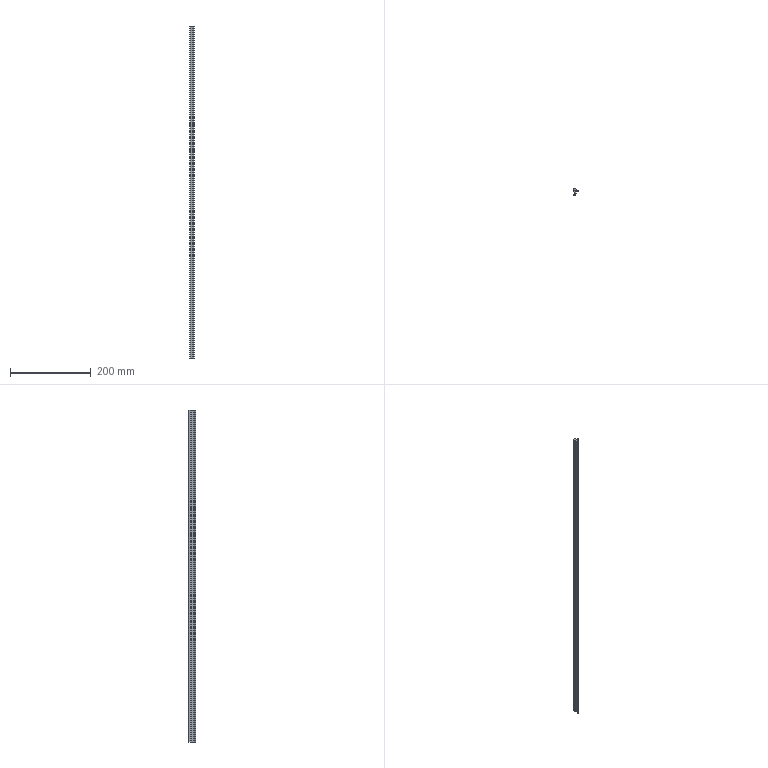Part | SolidWorks | features BaseBody 1, MoveFace 1 | 1 solid | 20 faces | box 10.8 x 17.5 x 820 mm | volume 64616 mm3 | cylinder 11 | plane 9 | commonest cylinder face diameters 1.6 x2 14 x2 0.4 x1 0.6 x1 0.8 x1 2.6 x1
STEP:
#1=CARTESIAN_POINT('',(-3.236,-11.055,720.));
#2=VERTEX_POINT('',#1);
#3=CARTESIAN_POINT('',(-4.3,-10.3,720.));
#4=VERTEX_POINT('',#3);
#5=CARTESIAN_POINT('',(-3.5,-10.3,720.));
#6=DIRECTION('',(0.,0.,-1.));
#7=DIRECTION('',(1.,0.,0.));
#8=AXIS2_PLACEMENT_3D('',#5,#6,#7);
#9=CIRCLE('',#8,0.8);
#10=EDGE_CURVE('',#2,#4,#9,.T.);
#11=ORIENTED_EDGE('',*,*,#10,.T.);
#12=CARTESIAN_POINT('',(-4.3,-10.3,-100.));
#13=VERTEX_POINT('',#12);
#14=CARTESIAN_POINT('',(-4.3,-10.3,-100.));
#15=DIRECTION('',(0.,0.,-1.));
#16=VECTOR('',#15,1000.);
#17=LINE('',#14,#16);
#18=EDGE_CURVE('',#4,#13,#17,.T.);
#19=ORIENTED_EDGE('',*,*,#18,.T.);
#20=CARTESIAN_POINT('',(-3.236,-11.055,-100.));
#21=VERTEX_POINT('',#20);
#22=CARTESIAN_POINT('',(-3.5,-10.3,-100.));
#23=DIRECTION('',(0.,0.,1.));
#24=DIRECTION('',(-1.,0.,0.));
#25=AXIS2_PLACEMENT_3D('',#22,#23,#24);
#26=CIRCLE('',#25,0.8);
#27=EDGE_CURVE('',#13,#21,#26,.T.);
#28=ORIENTED_EDGE('',*,*,#27,.T.);
#29=CARTESIAN_POINT('',(-3.236,-11.055,-100.));
#30=DIRECTION('',(0.,0.,-1.));
#31=VECTOR('',#30,1000.);
#32=LINE('',#29,#31);
#33=EDGE_CURVE('',#2,#21,#32,.T.);
#34=ORIENTED_EDGE('',*,*,#33,.F.);
#35=EDGE_LOOP('',(#11,#19,#28,#34));
#36=FACE_OUTER_BOUND('',#35,.T.);
#37=CARTESIAN_POINT('',(-3.5,-10.3,-100.));
#38=DIRECTION('',(0.,0.,-1.));
#39=DIRECTION('',(-1.,0.,0.));
#40=AXIS2_PLACEMENT_3D('',#37,#38,#39);
#41=CYLINDRICAL_SURFACE('',#40,0.8);
#42=ADVANCED_FACE('',(#36),#41,.T.);
#43=CARTESIAN_POINT('',(1.184,-6.397,-100.));
#44=VERTEX_POINT('',#43);
#45=CARTESIAN_POINT('',(-5.702,-4.29,-100.));
#46=DIRECTION('',(0.,0.,1.));
#47=DIRECTION('',(-1.,0.,0.));
#48=AXIS2_PLACEMENT_3D('',#45,#46,#47);
#49=CIRCLE('',#48,7.201);
#50=EDGE_CURVE('',#21,#44,#49,.T.);
#51=ORIENTED_EDGE('',*,*,#50,.T.);
#52=CARTESIAN_POINT('',(1.184,-6.397,720.));
#53=VERTEX_POINT('',#52);
#54=CARTESIAN_POINT('',(1.184,-6.397,-100.));
#55=DIRECTION('',(0.,0.,1.));
#56=VECTOR('',#55,1000.);
#57=LINE('',#54,#56);
#58=EDGE_CURVE('',#44,#53,#57,.T.);
#59=ORIENTED_EDGE('',*,*,#58,.T.);
#60=CARTESIAN_POINT('',(-5.702,-4.29,720.));
#61=DIRECTION('',(0.,0.,-1.));
#62=DIRECTION('',(1.,0.,0.));
#63=AXIS2_PLACEMENT_3D('',#60,#61,#62);
#64=CIRCLE('',#63,7.201);
#65=EDGE_CURVE('',#53,#2,#64,.T.);
#66=ORIENTED_EDGE('',*,*,#65,.T.);
#67=ORIENTED_EDGE('',*,*,#33,.T.);
#68=EDGE_LOOP('',(#51,#59,#66,#67));
#69=FACE_OUTER_BOUND('',#68,.T.);
#70=CARTESIAN_POINT('',(-5.702,-4.29,-100.));
#71=DIRECTION('',(0.,0.,-1.));
#72=DIRECTION('',(-1.,0.,0.));
#73=AXIS2_PLACEMENT_3D('',#70,#71,#72);
#74=CYLINDRICAL_SURFACE('',#73,7.201);
#75=ADVANCED_FACE('',(#69),#74,.T.);
#76=CARTESIAN_POINT('',(0.9,-6.,-100.));
#77=VERTEX_POINT('',#76);
#78=CARTESIAN_POINT('',(0.9,-6.3,-100.));
#79=DIRECTION('',(0.,0.,1.));
#80=DIRECTION('',(-1.,0.,0.));
#81=AXIS2_PLACEMENT_3D('',#78,#79,#80);
#82=CIRCLE('',#81,0.3);
#83=EDGE_CURVE('',#44,#77,#82,.T.);
#84=ORIENTED_EDGE('',*,*,#83,.T.);
#85=CARTESIAN_POINT('',(0.9,-6.,720.));
#86=VERTEX_POINT('',#85);
#87=CARTESIAN_POINT('',(0.9,-6.,-100.));
#88=DIRECTION('',(0.,0.,1.));
#89=VECTOR('',#88,1000.);
#90=LINE('',#87,#89);
#91=EDGE_CURVE('',#77,#86,#90,.T.);
#92=ORIENTED_EDGE('',*,*,#91,.T.);
#93=CARTESIAN_POINT('',(0.9,-6.3,720.));
#94=DIRECTION('',(0.,0.,-1.));
#95=DIRECTION('',(1.,0.,0.));
#96=AXIS2_PLACEMENT_3D('',#93,#94,#95);
#97=CIRCLE('',#96,0.3);
#98=EDGE_CURVE('',#86,#53,#97,.T.);
#99=ORIENTED_EDGE('',*,*,#98,.T.);
#100=ORIENTED_EDGE('',*,*,#58,.F.);
#101=EDGE_LOOP('',(#84,#92,#99,#100));
#102=FACE_OUTER_BOUND('',#101,.T.);
#103=CARTESIAN_POINT('',(0.9,-6.3,-100.));
#104=DIRECTION('',(0.,0.,-1.));
#105=DIRECTION('',(-1.,0.,0.));
#106=AXIS2_PLACEMENT_3D('',#103,#104,#105);
#107=CYLINDRICAL_SURFACE('',#106,0.3);
#108=ADVANCED_FACE('',(#102),#107,.T.);
#109=CARTESIAN_POINT('',(-2.5,-0.5,-100.));
#110=VERTEX_POINT('',#109);
#111=CARTESIAN_POINT('',(-2.5,-6.153,-100.));
#112=VERTEX_POINT('',#111);
#113=CARTESIAN_POINT('',(-2.5,-6.397,-100.));
#114=DIRECTION('',(0.,-1.,0.));
#115=VECTOR('',#114,1000.);
#116=LINE('',#113,#115);
#117=EDGE_CURVE('',#110,#112,#116,.T.);
#118=ORIENTED_EDGE('',*,*,#117,.F.);
#119=CARTESIAN_POINT('',(-4.2,1.695,-100.));
#120=VERTEX_POINT('',#119);
#121=CARTESIAN_POINT('',(-1.701,1.875,-100.));
#122=DIRECTION('',(0.,0.,1.));
#123=DIRECTION('',(-1.,0.,0.));
#124=AXIS2_PLACEMENT_3D('',#121,#122,#123);
#125=CIRCLE('',#124,2.506);
#126=EDGE_CURVE('',#120,#110,#125,.T.);
#127=ORIENTED_EDGE('',*,*,#126,.F.);
#128=CARTESIAN_POINT('',(-4.2,5.1,-100.));
#129=VERTEX_POINT('',#128);
#130=CARTESIAN_POINT('',(-4.2,-6.397,-100.));
#131=DIRECTION('',(0.,-1.,0.));
#132=VECTOR('',#131,1000.);
#133=LINE('',#130,#132);
#134=EDGE_CURVE('',#129,#120,#133,.T.);
#135=ORIENTED_EDGE('',*,*,#134,.F.);
#136=CARTESIAN_POINT('',(-2.892,6.4,-100.));
#137=VERTEX_POINT('',#136);
#138=CARTESIAN_POINT('',(-2.9,5.1,-100.));
#139=DIRECTION('',(0.,0.,1.));
#140=DIRECTION('',(-1.,0.,0.));
#141=AXIS2_PLACEMENT_3D('',#138,#139,#140);
#142=CIRCLE('',#141,1.3);
#143=EDGE_CURVE('',#137,#129,#142,.T.);
#144=ORIENTED_EDGE('',*,*,#143,.F.);
#145=CARTESIAN_POINT('',(0.5,5.5,-100.));
#146=VERTEX_POINT('',#145);
#147=CARTESIAN_POINT('',(-2.934,-0.5999,-100.));
#148=DIRECTION('',(0.,0.,1.));
#149=DIRECTION('',(-1.,0.,0.));
#150=AXIS2_PLACEMENT_3D('',#147,#148,#149);
#151=CIRCLE('',#150,7.);
#152=EDGE_CURVE('',#146,#137,#151,.T.);
#153=ORIENTED_EDGE('',*,*,#152,.F.);
#154=CARTESIAN_POINT('',(5.5,1.7,-100.));
#155=VERTEX_POINT('',#154);
#156=CARTESIAN_POINT('',(5.5,1.7,-100.));
#157=DIRECTION('',(-0.7962,0.6051,0.));
#158=VECTOR('',#157,1000.);
#159=LINE('',#156,#158);
#160=EDGE_CURVE('',#155,#146,#159,.T.);
#161=ORIENTED_EDGE('',*,*,#160,.F.);
#162=CARTESIAN_POINT('',(6.458,-0.2215,-100.));
#163=VERTEX_POINT('',#162);
#164=CARTESIAN_POINT('',(6.458,-0.2215,-100.));
#165=DIRECTION('',(-0.4462,0.8949,0.));
#166=VECTOR('',#165,1000.);
#167=LINE('',#164,#166);
#168=EDGE_CURVE('',#163,#155,#167,.T.);
#169=ORIENTED_EDGE('',*,*,#168,.F.);
#170=CARTESIAN_POINT('',(5.895,-0.7433,-100.));
#171=VERTEX_POINT('',#170);
#172=CARTESIAN_POINT('',(6.1,-0.4,-100.));
#173=DIRECTION('',(0.,0.,1.));
#174=DIRECTION('',(-1.,0.,0.));
#175=AXIS2_PLACEMENT_3D('',#172,#173,#174);
#176=CIRCLE('',#175,0.4);
#177=EDGE_CURVE('',#171,#163,#176,.T.);
#178=ORIENTED_EDGE('',*,*,#177,.F.);
#179=CARTESIAN_POINT('',(3.,0.,-100.));
#180=VERTEX_POINT('',#179);
#181=CARTESIAN_POINT('',(2.746,-6.995,-100.));
#182=DIRECTION('',(0.,0.,-1.));
#183=DIRECTION('',(-1.,0.,0.));
#184=AXIS2_PLACEMENT_3D('',#181,#182,#183);
#185=CIRCLE('',#184,7.);
#186=EDGE_CURVE('',#180,#171,#185,.T.);
#187=ORIENTED_EDGE('',*,*,#186,.F.);
#188=CARTESIAN_POINT('',(0.,0.,-100.));
#189=VERTEX_POINT('',#188);
#190=CARTESIAN_POINT('',(-6.814,0.,-100.));
#191=DIRECTION('',(1.,0.,0.));
#192=VECTOR('',#191,1000.);
#193=LINE('',#190,#192);
#194=EDGE_CURVE('',#189,#180,#193,.T.);
#195=ORIENTED_EDGE('',*,*,#194,.F.);
#196=CARTESIAN_POINT('',(0.,-5.8,-100.));
#197=VERTEX_POINT('',#196);
#198=CARTESIAN_POINT('',(0.,-6.397,-100.));
#199=DIRECTION('',(0.,1.,0.));
#200=VECTOR('',#199,1000.);
#201=LINE('',#198,#200);
#202=EDGE_CURVE('',#197,#189,#201,.T.);
#203=ORIENTED_EDGE('',*,*,#202,.F.);
#204=CARTESIAN_POINT('',(0.2,-6.,-100.));
#205=VERTEX_POINT('',#204);
#206=CARTESIAN_POINT('',(0.2,-5.8,-100.));
#207=DIRECTION('',(0.,0.,1.));
#208=DIRECTION('',(-1.,0.,0.));
#209=AXIS2_PLACEMENT_3D('',#206,#207,#208);
#210=CIRCLE('',#209,0.2);
#211=EDGE_CURVE('',#197,#205,#210,.T.);
#212=ORIENTED_EDGE('',*,*,#211,.T.);
#213=CARTESIAN_POINT('',(-6.814,-6.,-100.));
#214=DIRECTION('',(-1.,0.,0.));
#215=VECTOR('',#214,1000.);
#216=LINE('',#213,#215);
#217=EDGE_CURVE('',#77,#205,#216,.T.);
#218=ORIENTED_EDGE('',*,*,#217,.F.);
#219=ORIENTED_EDGE('',*,*,#83,.F.);
#220=ORIENTED_EDGE('',*,*,#50,.F.);
#221=ORIENTED_EDGE('',*,*,#27,.F.);
#222=CARTESIAN_POINT('',(-3.998,-9.674,-100.));
#223=VERTEX_POINT('',#222);
#224=CARTESIAN_POINT('',(-3.5,-10.3,-100.));
#225=DIRECTION('',(0.,0.,1.));
#226=DIRECTION('',(-1.,0.,0.));
#227=AXIS2_PLACEMENT_3D('',#224,#225,#226);
#228=CIRCLE('',#227,0.8);
#229=EDGE_CURVE('',#223,#13,#228,.T.);
#230=ORIENTED_EDGE('',*,*,#229,.F.);
#231=CARTESIAN_POINT('',(-6.814,-6.397,-100.));
#232=DIRECTION('',(0.,0.,-1.));
#233=DIRECTION('',(-1.,0.,0.));
#234=AXIS2_PLACEMENT_3D('',#231,#232,#233);
#235=CIRCLE('',#234,4.321);
#236=EDGE_CURVE('',#112,#223,#235,.T.);
#237=ORIENTED_EDGE('',*,*,#236,.F.);
#238=EDGE_LOOP('',(#118,#127,#135,#144,#153,#161,#169,#178,#187,#195,#203,#212,#218,#219,#220,#221,#230,#237));
#239=FACE_OUTER_BOUND('',#238,.T.);
#240=CARTESIAN_POINT('',(-6.814,-6.397,-100.));
#241=DIRECTION('',(0.,0.,1.));
#242=DIRECTION('',(1.,0.,0.));
#243=AXIS2_PLACEMENT_3D('',#240,#241,#242);
#244=PLANE('',#243);
#245=ADVANCED_FACE('',(#239),#244,.F.);
#246=ORIENTED_EDGE('',*,*,#18,.F.);
#247=CARTESIAN_POINT('',(-3.998,-9.674,720.));
#248=VERTEX_POINT('',#247);
#249=CARTESIAN_POINT('',(-3.5,-10.3,720.));
#250=DIRECTION('',(0.,0.,-1.));
#251=DIRECTION('',(1.,0.,0.));
#252=AXIS2_PLACEMENT_3D('',#249,#250,#251);
#253=CIRCLE('',#252,0.8);
#254=EDGE_CURVE('',#4,#248,#253,.T.);
#255=ORIENTED_EDGE('',*,*,#254,.T.);
#256=CARTESIAN_POINT('',(-3.998,-9.674,-100.));
#257=DIRECTION('',(0.,0.,-1.));
#258=VECTOR('',#257,1000.);
#259=LINE('',#256,#258);
#260=EDGE_CURVE('',#248,#223,#259,.T.);
#261=ORIENTED_EDGE('',*,*,#260,.T.);
#262=ORIENTED_EDGE('',*,*,#229,.T.);
#263=EDGE_LOOP('',(#246,#255,#261,#262));
#264=FACE_OUTER_BOUND('',#263,.T.);
#265=CARTESIAN_POINT('',(-3.5,-10.3,-100.));
#266=DIRECTION('',(0.,0.,-1.));
#267=DIRECTION('',(-1.,0.,0.));
#268=AXIS2_PLACEMENT_3D('',#265,#266,#267);
#269=CYLINDRICAL_SURFACE('',#268,0.8);
#270=ADVANCED_FACE('',(#264),#269,.T.);
#271=CARTESIAN_POINT('',(-4.2,1.695,720.));
#272=VERTEX_POINT('',#271);
#273=CARTESIAN_POINT('',(-2.5,-0.5,720.));
#274=VERTEX_POINT('',#273);
#275=CARTESIAN_POINT('',(-1.701,1.875,720.));
#276=DIRECTION('',(0.,0.,1.));
#277=DIRECTION('',(1.,0.,0.));
#278=AXIS2_PLACEMENT_3D('',#275,#276,#277);
#279=CIRCLE('',#278,2.506);
#280=EDGE_CURVE('',#272,#274,#279,.T.);
#281=ORIENTED_EDGE('',*,*,#280,.T.);
#282=CARTESIAN_POINT('',(-2.5,-6.153,720.));
#283=VERTEX_POINT('',#282);
#284=CARTESIAN_POINT('',(-2.5,-6.397,720.));
#285=DIRECTION('',(0.,-1.,0.));
#286=VECTOR('',#285,1000.);
#287=LINE('',#284,#286);
#288=EDGE_CURVE('',#274,#283,#287,.T.);
#289=ORIENTED_EDGE('',*,*,#288,.T.);
#290=CARTESIAN_POINT('',(-6.814,-6.397,720.));
#291=DIRECTION('',(0.,0.,-1.));
#292=DIRECTION('',(1.,0.,0.));
#293=AXIS2_PLACEMENT_3D('',#290,#291,#292);
#294=CIRCLE('',#293,4.321);
#295=EDGE_CURVE('',#283,#248,#294,.T.);
#296=ORIENTED_EDGE('',*,*,#295,.T.);
#297=ORIENTED_EDGE('',*,*,#254,.F.);
#298=ORIENTED_EDGE('',*,*,#10,.F.);
#299=ORIENTED_EDGE('',*,*,#65,.F.);
#300=ORIENTED_EDGE('',*,*,#98,.F.);
#301=CARTESIAN_POINT('',(0.2,-6.,720.));
#302=VERTEX_POINT('',#301);
#303=CARTESIAN_POINT('',(-6.814,-6.,720.));
#304=DIRECTION('',(-1.,0.,0.));
#305=VECTOR('',#304,1000.);
#306=LINE('',#303,#305);
#307=EDGE_CURVE('',#86,#302,#306,.T.);
#308=ORIENTED_EDGE('',*,*,#307,.T.);
#309=CARTESIAN_POINT('',(0.,-5.8,720.));
#310=VERTEX_POINT('',#309);
#311=CARTESIAN_POINT('',(0.2,-5.8,720.));
#312=DIRECTION('',(0.,0.,-1.));
#313=DIRECTION('',(1.,0.,0.));
#314=AXIS2_PLACEMENT_3D('',#311,#312,#313);
#315=CIRCLE('',#314,0.2);
#316=EDGE_CURVE('',#302,#310,#315,.T.);
#317=ORIENTED_EDGE('',*,*,#316,.T.);
#318=CARTESIAN_POINT('',(0.,0.,720.));
#319=VERTEX_POINT('',#318);
#320=CARTESIAN_POINT('',(0.,-6.397,720.));
#321=DIRECTION('',(0.,1.,0.));
#322=VECTOR('',#321,1000.);
#323=LINE('',#320,#322);
#324=EDGE_CURVE('',#310,#319,#323,.T.);
#325=ORIENTED_EDGE('',*,*,#324,.T.);
#326=CARTESIAN_POINT('',(3.,0.,720.));
#327=VERTEX_POINT('',#326);
#328=CARTESIAN_POINT('',(-6.814,0.,720.));
#329=DIRECTION('',(1.,0.,0.));
#330=VECTOR('',#329,1000.);
#331=LINE('',#328,#330);
#332=EDGE_CURVE('',#319,#327,#331,.T.);
#333=ORIENTED_EDGE('',*,*,#332,.T.);
#334=CARTESIAN_POINT('',(5.895,-0.7433,720.));
#335=VERTEX_POINT('',#334);
#336=CARTESIAN_POINT('',(2.746,-6.995,720.));
#337=DIRECTION('',(0.,0.,-1.));
#338=DIRECTION('',(1.,0.,0.));
#339=AXIS2_PLACEMENT_3D('',#336,#337,#338);
#340=CIRCLE('',#339,7.);
#341=EDGE_CURVE('',#327,#335,#340,.T.);
#342=ORIENTED_EDGE('',*,*,#341,.T.);
#343=CARTESIAN_POINT('',(6.458,-0.2215,720.));
#344=VERTEX_POINT('',#343);
#345=CARTESIAN_POINT('',(6.1,-0.4,720.));
#346=DIRECTION('',(0.,0.,-1.));
#347=DIRECTION('',(1.,0.,0.));
#348=AXIS2_PLACEMENT_3D('',#345,#346,#347);
#349=CIRCLE('',#348,0.4);
#350=EDGE_CURVE('',#344,#335,#349,.T.);
#351=ORIENTED_EDGE('',*,*,#350,.F.);
#352=CARTESIAN_POINT('',(5.5,1.7,720.));
#353=VERTEX_POINT('',#352);
#354=CARTESIAN_POINT('',(6.282,0.1323,720.));
#355=DIRECTION('',(-0.4462,0.8949,0.));
#356=VECTOR('',#355,1000.);
#357=LINE('',#354,#356);
#358=EDGE_CURVE('',#344,#353,#357,.T.);
#359=ORIENTED_EDGE('',*,*,#358,.T.);
#360=CARTESIAN_POINT('',(0.5,5.5,720.));
#361=VERTEX_POINT('',#360);
#362=CARTESIAN_POINT('',(1.595,4.668,720.));
#363=DIRECTION('',(-0.7962,0.6051,0.));
#364=VECTOR('',#363,1000.);
#365=LINE('',#362,#364);
#366=EDGE_CURVE('',#353,#361,#365,.T.);
#367=ORIENTED_EDGE('',*,*,#366,.T.);
#368=CARTESIAN_POINT('',(-2.892,6.4,720.));
#369=VERTEX_POINT('',#368);
#370=CARTESIAN_POINT('',(-2.934,-0.5999,720.));
#371=DIRECTION('',(0.,0.,1.));
#372=DIRECTION('',(1.,0.,0.));
#373=AXIS2_PLACEMENT_3D('',#370,#371,#372);
#374=CIRCLE('',#373,7.);
#375=EDGE_CURVE('',#361,#369,#374,.T.);
#376=ORIENTED_EDGE('',*,*,#375,.T.);
#377=CARTESIAN_POINT('',(-4.2,5.1,720.));
#378=VERTEX_POINT('',#377);
#379=CARTESIAN_POINT('',(-2.9,5.1,720.));
#380=DIRECTION('',(0.,0.,1.));
#381=DIRECTION('',(1.,0.,0.));
#382=AXIS2_PLACEMENT_3D('',#379,#380,#381);
#383=CIRCLE('',#382,1.3);
#384=EDGE_CURVE('',#369,#378,#383,.T.);
#385=ORIENTED_EDGE('',*,*,#384,.T.);
#386=CARTESIAN_POINT('',(-4.2,-6.397,720.));
#387=DIRECTION('',(0.,-1.,0.));
#388=VECTOR('',#387,1000.);
#389=LINE('',#386,#388);
#390=EDGE_CURVE('',#378,#272,#389,.T.);
#391=ORIENTED_EDGE('',*,*,#390,.T.);
#392=EDGE_LOOP('',(#281,#289,#296,#297,#298,#299,#300,#308,#317,#325,#333,#342,#351,#359,#367,#376,#385,#391));
#393=FACE_OUTER_BOUND('',#392,.T.);
#394=CARTESIAN_POINT('',(-6.814,-6.397,720.));
#395=DIRECTION('',(0.,0.,1.));
#396=DIRECTION('',(1.,0.,0.));
#397=AXIS2_PLACEMENT_3D('',#394,#395,#396);
#398=PLANE('',#397);
#399=ADVANCED_FACE('',(#393),#398,.T.);
#400=ORIENTED_EDGE('',*,*,#217,.T.);
#401=CARTESIAN_POINT('',(0.2,-6.,-100.));
#402=DIRECTION('',(0.,0.,1.));
#403=VECTOR('',#402,1000.);
#404=LINE('',#401,#403);
#405=EDGE_CURVE('',#205,#302,#404,.T.);
#406=ORIENTED_EDGE('',*,*,#405,.T.);
#407=ORIENTED_EDGE('',*,*,#307,.F.);
#408=ORIENTED_EDGE('',*,*,#91,.F.);
#409=EDGE_LOOP('',(#400,#406,#407,#408));
#410=FACE_OUTER_BOUND('',#409,.T.);
#411=CARTESIAN_POINT('',(0.9,-6.,-100.));
#412=DIRECTION('',(0.,1.,0.));
#413=DIRECTION('',(0.,0.,1.));
#414=AXIS2_PLACEMENT_3D('',#411,#412,#413);
#415=PLANE('',#414);
#416=ADVANCED_FACE('',(#410),#415,.T.);
#417=CARTESIAN_POINT('',(-2.5,-6.153,-100.));
#418=DIRECTION('',(0.,0.,1.));
#419=VECTOR('',#418,1000.);
#420=LINE('',#417,#419);
#421=EDGE_CURVE('',#112,#283,#420,.T.);
#422=ORIENTED_EDGE('',*,*,#421,.F.);
#423=ORIENTED_EDGE('',*,*,#236,.T.);
#424=ORIENTED_EDGE('',*,*,#260,.F.);
#425=ORIENTED_EDGE('',*,*,#295,.F.);
#426=EDGE_LOOP('',(#422,#423,#424,#425));
#427=FACE_OUTER_BOUND('',#426,.T.);
#428=CARTESIAN_POINT('',(-6.814,-6.397,-100.));
#429=DIRECTION('',(0.,0.,-1.));
#430=DIRECTION('',(-1.,0.,0.));
#431=AXIS2_PLACEMENT_3D('',#428,#429,#430);
#432=CYLINDRICAL_SURFACE('',#431,4.321);
#433=ADVANCED_FACE('',(#427),#432,.F.);
#434=ORIENTED_EDGE('',*,*,#117,.T.);
#435=ORIENTED_EDGE('',*,*,#421,.T.);
#436=ORIENTED_EDGE('',*,*,#288,.F.);
#437=CARTESIAN_POINT('',(-2.5,-0.5,-100.));
#438=DIRECTION('',(0.,0.,-1.));
#439=VECTOR('',#438,1000.);
#440=LINE('',#437,#439);
#441=EDGE_CURVE('',#274,#110,#440,.T.);
#442=ORIENTED_EDGE('',*,*,#441,.T.);
#443=EDGE_LOOP('',(#434,#435,#436,#442));
#444=FACE_OUTER_BOUND('',#443,.T.);
#445=CARTESIAN_POINT('',(-2.5,-0.5,-100.));
#446=DIRECTION('',(-1.,0.,0.));
#447=DIRECTION('',(0.,0.,1.));
#448=AXIS2_PLACEMENT_3D('',#445,#446,#447);
#449=PLANE('',#448);
#450=ADVANCED_FACE('',(#444),#449,.T.);
#451=ORIENTED_EDGE('',*,*,#126,.T.);
#452=ORIENTED_EDGE('',*,*,#441,.F.);
#453=ORIENTED_EDGE('',*,*,#280,.F.);
#454=CARTESIAN_POINT('',(-4.2,1.695,-100.));
#455=DIRECTION('',(0.,0.,-1.));
#456=VECTOR('',#455,1000.);
#457=LINE('',#454,#456);
#458=EDGE_CURVE('',#272,#120,#457,.T.);
#459=ORIENTED_EDGE('',*,*,#458,.T.);
#460=EDGE_LOOP('',(#451,#452,#453,#459));
#461=FACE_OUTER_BOUND('',#460,.T.);
#462=CARTESIAN_POINT('',(-1.701,1.875,-100.));
#463=DIRECTION('',(0.,0.,-1.));
#464=DIRECTION('',(-1.,0.,0.));
#465=AXIS2_PLACEMENT_3D('',#462,#463,#464);
#466=CYLINDRICAL_SURFACE('',#465,2.506);
#467=ADVANCED_FACE('',(#461),#466,.T.);
#468=ORIENTED_EDGE('',*,*,#134,.T.);
#469=ORIENTED_EDGE('',*,*,#458,.F.);
#470=ORIENTED_EDGE('',*,*,#390,.F.);
#471=CARTESIAN_POINT('',(-4.2,5.1,-100.));
#472=DIRECTION('',(0.,0.,-1.));
#473=VECTOR('',#472,1000.);
#474=LINE('',#471,#473);
#475=EDGE_CURVE('',#378,#129,#474,.T.);
#476=ORIENTED_EDGE('',*,*,#475,.T.);
#477=EDGE_LOOP('',(#468,#469,#470,#476));
#478=FACE_OUTER_BOUND('',#477,.T.);
#479=CARTESIAN_POINT('',(-4.2,5.1,-100.));
#480=DIRECTION('',(-1.,0.,0.));
#481=DIRECTION('',(0.,0.,1.));
#482=AXIS2_PLACEMENT_3D('',#479,#480,#481);
#483=PLANE('',#482);
#484=ADVANCED_FACE('',(#478),#483,.T.);
#485=ORIENTED_EDGE('',*,*,#143,.T.);
#486=ORIENTED_EDGE('',*,*,#475,.F.);
#487=ORIENTED_EDGE('',*,*,#384,.F.);
#488=CARTESIAN_POINT('',(-2.892,6.4,-100.));
#489=DIRECTION('',(0.,0.,-1.));
#490=VECTOR('',#489,1000.);
#491=LINE('',#488,#490);
#492=EDGE_CURVE('',#369,#137,#491,.T.);
#493=ORIENTED_EDGE('',*,*,#492,.T.);
#494=EDGE_LOOP('',(#485,#486,#487,#493));
#495=FACE_OUTER_BOUND('',#494,.T.);
#496=CARTESIAN_POINT('',(-2.9,5.1,-100.));
#497=DIRECTION('',(0.,0.,-1.));
#498=DIRECTION('',(-1.,0.,0.));
#499=AXIS2_PLACEMENT_3D('',#496,#497,#498);
#500=CYLINDRICAL_SURFACE('',#499,1.3);
#501=ADVANCED_FACE('',(#495),#500,.T.);
#502=ORIENTED_EDGE('',*,*,#152,.T.);
#503=ORIENTED_EDGE('',*,*,#492,.F.);
#504=ORIENTED_EDGE('',*,*,#375,.F.);
#505=CARTESIAN_POINT('',(0.5,5.5,-100.));
#506=DIRECTION('',(0.,0.,-1.));
#507=VECTOR('',#506,1000.);
#508=LINE('',#505,#507);
#509=EDGE_CURVE('',#361,#146,#508,.T.);
#510=ORIENTED_EDGE('',*,*,#509,.T.);
#511=EDGE_LOOP('',(#502,#503,#504,#510));
#512=FACE_OUTER_BOUND('',#511,.T.);
#513=CARTESIAN_POINT('',(-2.934,-0.5999,-100.));
#514=DIRECTION('',(0.,0.,-1.));
#515=DIRECTION('',(-1.,0.,0.));
#516=AXIS2_PLACEMENT_3D('',#513,#514,#515);
#517=CYLINDRICAL_SURFACE('',#516,7.);
#518=ADVANCED_FACE('',(#512),#517,.T.);
#519=ORIENTED_EDGE('',*,*,#160,.T.);
#520=ORIENTED_EDGE('',*,*,#509,.F.);
#521=ORIENTED_EDGE('',*,*,#366,.F.);
#522=CARTESIAN_POINT('',(5.5,1.7,-100.));
#523=DIRECTION('',(0.,0.,-1.));
#524=VECTOR('',#523,1000.);
#525=LINE('',#522,#524);
#526=EDGE_CURVE('',#353,#155,#525,.T.);
#527=ORIENTED_EDGE('',*,*,#526,.T.);
#528=EDGE_LOOP('',(#519,#520,#521,#527));
#529=FACE_OUTER_BOUND('',#528,.T.);
#530=CARTESIAN_POINT('',(5.5,1.7,-100.));
#531=DIRECTION('',(0.6051,0.7962,0.));
#532=DIRECTION('',(-0.7962,0.6051,0.));
#533=AXIS2_PLACEMENT_3D('',#530,#531,#532);
#534=PLANE('',#533);
#535=ADVANCED_FACE('',(#529),#534,.T.);
#536=ORIENTED_EDGE('',*,*,#168,.T.);
#537=ORIENTED_EDGE('',*,*,#526,.F.);
#538=ORIENTED_EDGE('',*,*,#358,.F.);
#539=CARTESIAN_POINT('',(6.458,-0.2215,-100.));
#540=DIRECTION('',(0.,0.,-1.));
#541=VECTOR('',#540,1000.);
#542=LINE('',#539,#541);
#543=EDGE_CURVE('',#344,#163,#542,.T.);
#544=ORIENTED_EDGE('',*,*,#543,.T.);
#545=EDGE_LOOP('',(#536,#537,#538,#544));
#546=FACE_OUTER_BOUND('',#545,.T.);
#547=CARTESIAN_POINT('',(6.458,-0.2215,-100.));
#548=DIRECTION('',(0.8949,0.4462,0.));
#549=DIRECTION('',(-0.4462,0.8949,0.));
#550=AXIS2_PLACEMENT_3D('',#547,#548,#549);
#551=PLANE('',#550);
#552=ADVANCED_FACE('',(#546),#551,.T.);
#553=CARTESIAN_POINT('',(3.,0.,-100.));
#554=DIRECTION('',(0.,0.,1.));
#555=VECTOR('',#554,1000.);
#556=LINE('',#553,#555);
#557=EDGE_CURVE('',#180,#327,#556,.T.);
#558=ORIENTED_EDGE('',*,*,#557,.F.);
#559=ORIENTED_EDGE('',*,*,#186,.T.);
#560=CARTESIAN_POINT('',(5.895,-0.7433,-100.));
#561=DIRECTION('',(0.,0.,-1.));
#562=VECTOR('',#561,1000.);
#563=LINE('',#560,#562);
#564=EDGE_CURVE('',#335,#171,#563,.T.);
#565=ORIENTED_EDGE('',*,*,#564,.F.);
#566=ORIENTED_EDGE('',*,*,#341,.F.);
#567=EDGE_LOOP('',(#558,#559,#565,#566));
#568=FACE_OUTER_BOUND('',#567,.T.);
#569=CARTESIAN_POINT('',(2.746,-6.995,-100.));
#570=DIRECTION('',(0.,0.,-1.));
#571=DIRECTION('',(-1.,0.,0.));
#572=AXIS2_PLACEMENT_3D('',#569,#570,#571);
#573=CYLINDRICAL_SURFACE('',#572,7.);
#574=ADVANCED_FACE('',(#568),#573,.F.);
#575=ORIENTED_EDGE('',*,*,#194,.T.);
#576=ORIENTED_EDGE('',*,*,#557,.T.);
#577=ORIENTED_EDGE('',*,*,#332,.F.);
#578=CARTESIAN_POINT('',(0.,0.,-100.));
#579=DIRECTION('',(0.,0.,-1.));
#580=VECTOR('',#579,1000.);
#581=LINE('',#578,#580);
#582=EDGE_CURVE('',#319,#189,#581,.T.);
#583=ORIENTED_EDGE('',*,*,#582,.T.);
#584=EDGE_LOOP('',(#575,#576,#577,#583));
#585=FACE_OUTER_BOUND('',#584,.T.);
#586=CARTESIAN_POINT('',(0.,0.,-100.));
#587=DIRECTION('',(0.,-1.,0.));
#588=DIRECTION('',(0.,0.,-1.));
#589=AXIS2_PLACEMENT_3D('',#586,#587,#588);
#590=PLANE('',#589);
#591=ADVANCED_FACE('',(#585),#590,.T.);
#592=ORIENTED_EDGE('',*,*,#202,.T.);
#593=ORIENTED_EDGE('',*,*,#582,.F.);
#594=ORIENTED_EDGE('',*,*,#324,.F.);
#595=CARTESIAN_POINT('',(0.,-5.8,-100.));
#596=DIRECTION('',(0.,0.,-1.));
#597=VECTOR('',#596,1000.);
#598=LINE('',#595,#597);
#599=EDGE_CURVE('',#310,#197,#598,.T.);
#600=ORIENTED_EDGE('',*,*,#599,.T.);
#601=EDGE_LOOP('',(#592,#593,#594,#600));
#602=FACE_OUTER_BOUND('',#601,.T.);
#603=CARTESIAN_POINT('',(0.,-5.8,-100.));
#604=DIRECTION('',(1.,0.,0.));
#605=DIRECTION('',(0.,0.,-1.));
#606=AXIS2_PLACEMENT_3D('',#603,#604,#605);
#607=PLANE('',#606);
#608=ADVANCED_FACE('',(#602),#607,.T.);
#609=ORIENTED_EDGE('',*,*,#405,.F.);
#610=ORIENTED_EDGE('',*,*,#211,.F.);
#611=ORIENTED_EDGE('',*,*,#599,.F.);
#612=ORIENTED_EDGE('',*,*,#316,.F.);
#613=EDGE_LOOP('',(#609,#610,#611,#612));
#614=FACE_OUTER_BOUND('',#613,.T.);
#615=CARTESIAN_POINT('',(0.2,-5.8,-100.));
#616=DIRECTION('',(0.,0.,-1.));
#617=DIRECTION('',(-1.,0.,0.));
#618=AXIS2_PLACEMENT_3D('',#615,#616,#617);
#619=CYLINDRICAL_SURFACE('',#618,0.2);
#620=ADVANCED_FACE('',(#614),#619,.F.);
#621=ORIENTED_EDGE('',*,*,#177,.T.);
#622=ORIENTED_EDGE('',*,*,#543,.F.);
#623=ORIENTED_EDGE('',*,*,#350,.T.);
#624=ORIENTED_EDGE('',*,*,#564,.T.);
#625=EDGE_LOOP('',(#621,#622,#623,#624));
#626=FACE_OUTER_BOUND('',#625,.T.);
#627=CARTESIAN_POINT('',(6.1,-0.4,-100.));
#628=DIRECTION('',(0.,0.,-1.));
#629=DIRECTION('',(-1.,0.,0.));
#630=AXIS2_PLACEMENT_3D('',#627,#628,#629);
#631=CYLINDRICAL_SURFACE('',#630,0.4);
#632=ADVANCED_FACE('',(#626),#631,.T.);
#633=CLOSED_SHELL('',(#42,#75,#108,#245,#270,#399,#416,#433,#450,#467,#484,#501,#518,#535,#552,#574,#591,#608,#620,#632));
#634=MANIFOLD_SOLID_BREP('',#633);
#635=CARTESIAN_POINT('',(0.,0.,0.));
#636=DIRECTION('',(0.,0.,1.));
#637=DIRECTION('',(1.,0.,0.));
#638=AXIS2_PLACEMENT_3D('',#635,#636,#637);
#639=(LENGTH_UNIT()NAMED_UNIT(*)SI_UNIT(.MILLI.,.METRE.));
#640=UNCERTAINTY_MEASURE_WITH_UNIT(LENGTH_MEASURE(0.00001),#639,'','');
#641=(NAMED_UNIT(*)PLANE_ANGLE_UNIT()SI_UNIT($,.RADIAN.));
#642=(NAMED_UNIT(*)SI_UNIT($,.STERADIAN.)SOLID_ANGLE_UNIT());
#643=(GEOMETRIC_REPRESENTATION_CONTEXT(3)GLOBAL_UNCERTAINTY_ASSIGNED_CONTEXT((#640))GLOBAL_UNIT_ASSIGNED_CONTEXT((#639,#641,#642))REPRESENTATION_CONTEXT('',''));
#644=ADVANCED_BREP_SHAPE_REPRESENTATION('',(#634,#638),#643);